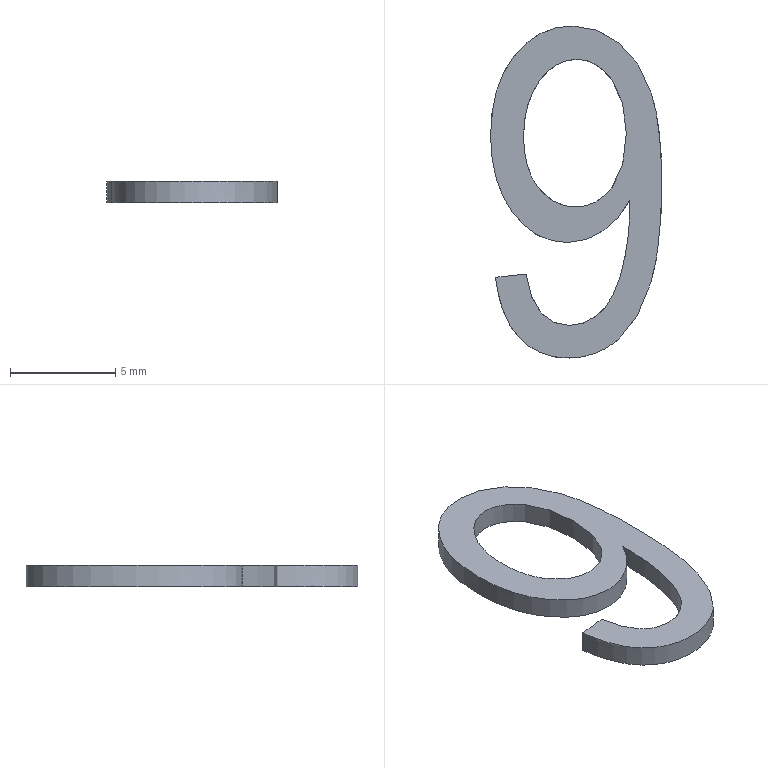Part | STEP file | lll_id1394_x_t | 1 solid | 4 faces | box 8.119 x 15.752 x 1 mm | volume 59.744 mm3 | other 2 | plane 2